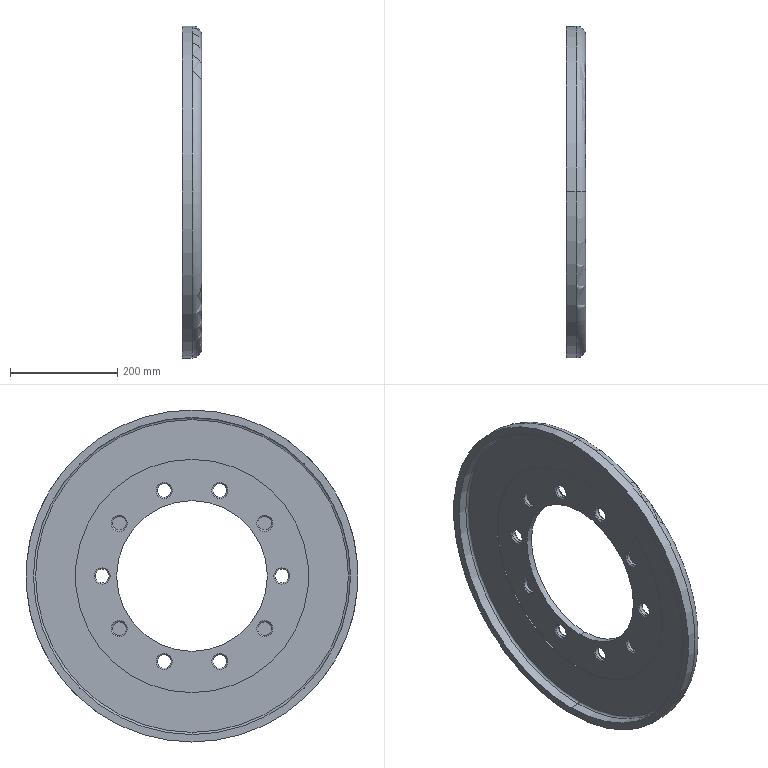Part | SolidWorks | features Fillet 2, Chamfer 1, CirPattern 1, ICE 1, RevCut 1, Revolution 1 | 1 solid | 86 faces | box 36 x 619 x 619 mm | volume 3559347 mm3 | cylinder 28 | sphere 20 | cone 20 | plane 14 | torus 4 | commonest cylinder face diameters 26 x20 281 x2 435 x2 591 x2 619 x2